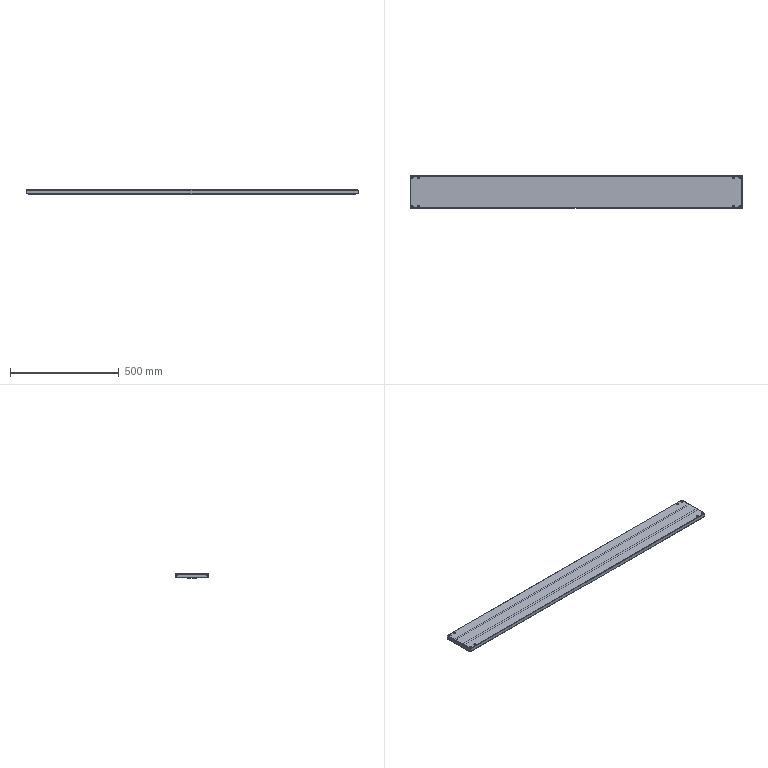Part | SolidWorks | 10 solids | 192 faces | box 1530 x 150 x 22 mm | volume 923330 mm3 | plane 128 | cylinder 56 | spline 8 | commonest cylinder face diameters 5 x16 8 x16 0.4 x12 4.4 x12